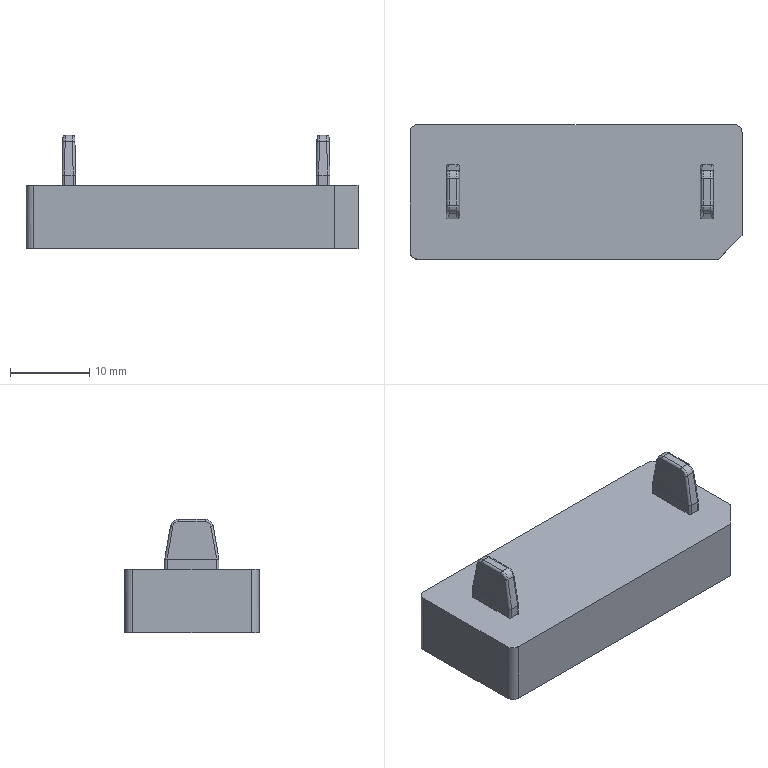NC program | PowerMill | posted by the shop | part box 42 x 17 x 14.346 mm
Lines 1 to 1529 of 50900:
%
G40 G49 G17 G80
( TOOL ID   D10C_1_1 )
( TOOL DIA. 10. TIP RAD 0 LENGTH 69.8 )
( Z = -.204 )
T1 M6
T3
G91 G28 Z0
G0 G90 G54
M08
S8000 M3
G0 X0 Y0 M8
G43 Z10.2 H1
X28.65 Y11.15
Z1.198
G1 Z-.002 F6000
X23.65 F10000
X-23.65
Y5.575
X23.65
Y0
X-23.65
Y-5.575
X23.65
Y-11.15
X-23.65
X-28.65
Z-.204
X-23.65
X23.65
Y-5.575
X-23.65
Y0
X23.65
Y5.575
X-23.65
Y11.15
X23.65
X28.65
G0 Z10.2
X.5 Y0
Z9.796
X-29.349 Y-4.749
Z.562
G1 Z-.638 F6000
X-28.822 F10000
G3 X-24.074 Y-.001 I0 J4.747
G1 Y10.15
G2 X-23.074 Y11.15 I1. J0
G1 X24.074
G2 X25.074 Y10.15 I0 J-1.
G1 Y-.001
X22.484 Y0
Y-2.32
X22.396 Y-3.094
X22.199 Y-3.867
X21.769 Y-4.832
X21.395 Y-5.414
X20.996 Y-5.89
X20.691 Y-6.187
X20.222 Y-6.578
X19.621 Y-6.961
X19.449 Y-7.051
X18.676 Y-7.361
X17.902 Y-7.548
X17.129 Y-7.619
X15.582 Y-7.593
X14.808 Y-7.454
X14.035 Y-7.199
X13.539 Y-6.961
X13.262 Y-6.798
X12.488 Y-6.204
X11.765 Y-5.414
X11.292 Y-4.641
X10.961 Y-3.867
X10.763 Y-3.094
X10.676 Y-2.32
Y-.093
X4.957 Y-.038
X4.925 Y-3.441
G2 X2.91 Y-5.422 I-2. J.019
G1 X-2.008 Y-5.386
G2 X-3.993 Y-3.373 I.014 J2.
G1 X-3.949 Y3.423
G2 X-1.938 Y5.409 I2. J-.013
G1 X3. Y5.383
G2 X4.989 Y3.364 I-.011 J-2.
G1 X4.957 Y-.038
X10.676 Y-.093
X10.675 Y2.32
X10.758 Y3.094
X10.941 Y3.849
X11.272 Y4.641
X11.715 Y5.385
X12.427 Y6.187
X13.262 Y6.838
X14.035 Y7.238
X14.808 Y7.493
X15.582 Y7.632
X17.129 Y7.659
X17.902 Y7.588
X18.676 Y7.401
X19.449 Y7.091
X19.692 Y6.961
X20.222 Y6.617
X20.733 Y6.187
X20.996 Y5.93
X21.424 Y5.414
X21.769 Y4.87
X21.888 Y4.641
X22.212 Y3.867
X22.402 Y3.094
X22.485 Y2.32
X22.484 Y0
X25.074 Y-.001
Y-10.15
G2 X24.074 Y-11.15 I-1. J0
G1 X-23.074
G2 X-24.074 Y-10.15 I0 J1.
G1 Y-.001
X-21.485 Y0
X-21.486 Y2.32
X-21.403 Y3.094
X-21.212 Y3.867
X-20.887 Y4.641
X-20.769 Y4.87
X-20.424 Y5.414
X-19.996 Y5.93
X-19.733 Y6.187
X-19.222 Y6.617
X-18.692 Y6.961
X-18.449 Y7.091
X-17.676 Y7.401
X-16.902 Y7.588
X-16.129 Y7.659
X-14.582 Y7.632
X-13.808 Y7.493
X-13.035 Y7.238
X-12.262 Y6.838
X-11.488 Y6.244
X-10.736 Y5.414
X-10.272 Y4.641
X-9.947 Y3.867
X-9.758 Y3.094
X-9.675 Y2.32
X-9.677 Y-2.32
X-9.763 Y-3.094
X-9.941 Y-3.809
X-10.292 Y-4.641
X-10.715 Y-5.346
X-11.469 Y-6.187
X-12.262 Y-6.798
X-12.538 Y-6.961
X-13.035 Y-7.198
X-13.808 Y-7.454
X-14.582 Y-7.593
X-16.129 Y-7.619
X-16.902 Y-7.548
X-17.676 Y-7.361
X-18.449 Y-7.051
X-19.222 Y-6.578
X-19.69 Y-6.187
X-19.996 Y-5.89
X-20.395 Y-5.414
X-20.769 Y-4.832
X-21.199 Y-3.867
X-21.397 Y-3.094
X-21.484 Y-2.32
X-21.485 Y0
X-24.074 Y-.001
G0 Z3.228
G1 X-29.349 Y-4.749
G0 Z.178
G1 Z-1.022 F6000
X-28.822 F10000
G3 X-24.074 Y-.001 I0 J4.747
G1 Y10.15
G2 X-23.074 Y11.15 I1. J0
G1 X24.074
G2 X25.074 Y10.15 I0 J-1.
G1 Y0
X22.5
Y-2.32
X22.445 Y-3.094
X22.283 Y-3.867
X21.995 Y-4.641
X21.769 Y-5.069
X21.553 Y-5.414
X20.996 Y-6.113
X20.222 Y-6.779
X19.954 Y-6.961
X19.449 Y-7.248
X18.676 Y-7.556
X17.924 Y-7.734
X17.129 Y-7.808
X15.582 Y-7.782
X14.808 Y-7.645
X14.035 Y-7.395
X13.262 Y-6.997
X12.488 Y-6.425
X12.237 Y-6.187
X11.715 Y-5.57
X11.165 Y-4.641
X10.877 Y-3.867
X10.715 Y-3.094
X10.66 Y-2.32
Y-.048
X4.896 Y-.019
X4.879 Y-3.412
G2 X2.879 Y-5.401 I-2. J.01
G1 X-1.878 Y-5.402
G2 X-3.878 Y-3.412 I0 J2.
G1 X-3.913 Y3.373
G2 X-1.913 Y5.383 I2. J.01
G1 X2.913
G2 X4.913 Y3.373 I0 J-2.
G1 X4.896 Y-.019
X10.66 Y-.048
X10.659 Y2.32
X10.709 Y3.094
X10.868 Y3.867
X10.941 Y4.117
X11.147 Y4.641
X11.581 Y5.414
X11.715 Y5.609
X12.199 Y6.187
X12.488 Y6.464
X13.142 Y6.961
X14.035 Y7.434
X14.808 Y7.684
X15.582 Y7.821
X17.129 Y7.847
X17.902 Y7.777
X18.676 Y7.596
X19.449 Y7.287
X20.222 Y6.821
X20.961 Y6.187
X21.579 Y5.414
X21.769 Y5.113
X22.013 Y4.641
X22.292 Y3.867
X22.452 Y3.094
X22.5 Y2.32
Y0
X25.074
Y-10.15
G2 X24.074 Y-11.15 I-1. J0
G1 X-23.074
G2 X-24.074 Y-10.15 I0 J1.
G1 Y-2.32
X-21.501
Y2.32
X-21.451 Y3.094
X-21.294 Y3.867
X-21.013 Y4.641
X-20.769 Y5.113
X-20.579 Y5.414
X-19.996 Y6.152
X-19.222 Y6.821
X-18.449 Y7.287
X-17.676 Y7.596
X-16.902 Y7.777
X-16.129 Y7.847
X-14.582 Y7.821
X-13.808 Y7.684
X-13.035 Y7.434
X-12.262 Y7.036
X-11.488 Y6.464
X-11.199 Y6.187
X-10.715 Y5.609
X-10.581 Y5.414
X-10.147 Y4.641
X-9.941 Y4.117
X-9.868 Y3.867
X-9.708 Y3.094
X-9.66 Y2.32
Y-2.32
X-9.715 Y-3.094
X-9.877 Y-3.867
X-10.165 Y-4.641
X-10.715 Y-5.57
X-11.237 Y-6.187
X-11.488 Y-6.425
X-12.206 Y-6.961
X-13.035 Y-7.395
X-13.808 Y-7.645
X-14.237 Y-7.734
X-14.582 Y-7.782
X-16.129 Y-7.808
X-16.902 Y-7.737
X-17.676 Y-7.556
X-18.449 Y-7.248
X-18.954 Y-6.961
X-19.222 Y-6.779
X-19.923 Y-6.187
X-20.553 Y-5.414
X-20.769 Y-5.069
X-20.995 Y-4.641
X-21.283 Y-3.867
X-21.446 Y-3.094
X-21.501 Y-2.32
X-24.074
Y-.001
G0 Z2.844
G1 X-29.349 Y-4.749
G0 Z-.206
G1 Z-1.406 F6000
X-28.822 F10000
G3 X-24.074 Y-.001 I0 J4.747
G1 Y10.15
G2 X-23.074 Y11.15 I1. J0
G1 X24.074
G2 X25.074 Y10.15 I0 J-1.
G1 Y0
X22.507
Y-2.32
X22.463 Y-3.094
X22.303 Y-3.867
X22.036 Y-4.641
X21.769 Y-5.167
X21.616 Y-5.414
X20.991 Y-6.187
X20.222 Y-6.866
X19.449 Y-7.327
X18.676 Y-7.627
X18.278 Y-7.734
X17.902 Y-7.812
X17.129 Y-7.881
X15.582 Y-7.855
X14.881 Y-7.734
X14.035 Y-7.47
X13.262 Y-7.081
X13.074 Y-6.961
X12.488 Y-6.501
X12.169 Y-6.187
X11.715 Y-5.657
X11.544 Y-5.414
X11.124 Y-4.641
X10.856 Y-3.867
X10.697 Y-3.094
X10.653 Y-2.32
Y2.32
X10.692 Y3.094
X10.846 Y3.867
X10.941 Y4.198
X11.108 Y4.641
X11.518 Y5.414
X11.715 Y5.697
X12.13 Y6.187
X12.488 Y6.54
X13.018 Y6.961
X13.262 Y7.121
X14.035 Y7.509
X14.731 Y7.734
X15.582 Y7.894
X17.129 Y7.92
X17.902 Y7.851
X18.676 Y7.666
X19.449 Y7.366
X20.142 Y6.961
X20.996 Y6.222
X21.641 Y5.414
X21.769 Y5.207
X22.053 Y4.641
X22.314 Y3.867
X22.467 Y3.094
X22.507 Y2.32
Y0
X25.074
Y-10.15
G2 X24.074 Y-11.15 I-1. J0
G1 X-23.074
G2 X-24.074 Y-10.15 I0 J1.
G1 Y-2.757
X-21.491 Y-2.61
X-21.507 Y-2.32
Y2.32
X-21.468 Y3.094
X-21.314 Y3.867
X-21.053 Y4.641
X-20.769 Y5.207
X-20.642 Y5.414
X-20.03 Y6.187
X-19.222 Y6.905
X-18.449 Y7.366
X-17.676 Y7.666
X-16.902 Y7.851
X-16.129 Y7.92
X-14.582 Y7.894
X-13.808 Y7.755
X-13.035 Y7.509
X-12.262 Y7.121
X-12.018 Y6.961
X-11.488 Y6.54
X-11.131 Y6.187
X-10.715 Y5.697
X-10.519 Y5.414
X-10.107 Y4.641
X-9.941 Y4.198
X-9.846 Y3.867
X-9.692 Y3.094
X-9.653 Y2.32
Y.002
X-3.902 Y-.001
X-3.901 Y3.379
G2 X-1.901 Y5.378 I2. J-.001
G1 X2.901 Y5.377
G2 X4.901 Y3.379 I0 J-2.
G1 X4.904 Y-3.38
G2 X2.904 Y-5.381 I-2. J-.001
G1 X-1.904
G2 X-3.904 Y-3.38 I0 J2.
G1 X-3.902 Y-.001
X-9.653 Y.002
Y-2.32
X-9.697 Y-3.094
X-9.856 Y-3.867
X-9.941 Y-4.159
X-10.124 Y-4.641
X-10.544 Y-5.414
X-10.715 Y-5.657
X-11.169 Y-6.187
X-11.488 Y-6.501
X-12.075 Y-6.961
X-12.262 Y-7.081
X-13.035 Y-7.47
X-13.882 Y-7.734
X-14.582 Y-7.855
X-16.129 Y-7.881
X-16.902 Y-7.812
X-17.676 Y-7.627
X-18.449 Y-7.327
X-19.222 Y-6.866
X-19.992 Y-6.187
X-20.617 Y-5.414
X-20.769 Y-5.167
X-21.036 Y-4.641
X-21.303 Y-3.867
X-21.463 Y-3.094
X-21.491 Y-2.61
X-24.074 Y-2.757
Y-.001
G0 Z2.459
G1 X-29.349 Y-4.749
G0 Z-.591
G1 Z-1.791 F6000
X-28.822 F10000
G3 X-24.074 Y-.001 I0 J4.747
G1 Y0
X-21.514
Y2.32
X-21.482 Y3.094
X-21.337 Y3.867
X-21.088 Y4.641
X-20.769 Y5.286
X-20.099 Y6.187
X-19.245 Y6.961
X-18.449 Y7.437
X-17.68 Y7.734
X-16.902 Y7.92
X-16.129 Y7.988
X-14.582 Y7.963
X-13.808 Y7.825
X-13.035 Y7.58
X-12.262 Y7.192
X-11.916 Y6.961
X-11.488 Y6.614
X-11.06 Y6.187
X-10.715 Y5.774
X-10.469 Y5.414
X-10.072 Y4.641
X-9.941 Y4.286
X-9.822 Y3.867
X-9.677 Y3.094
X-9.646 Y2.32
Y-.027
X-3.879 Y-.013
X-3.887 Y3.366
G2 X-1.892 Y5.371 I2. J.005
G1 X2.862 Y5.383
G2 X4.867 Y3.39 I.005 J-2.
G1 X4.891 Y-3.368
G2 X2.897 Y-5.375 I-2. J-.007
G1 X-1.865 Y-5.388
G2 X-3.871 Y-3.392 I-.005 J2.
G1 X-3.879 Y-.013
X-9.646 Y-.027
Y-2.32
X-9.682 Y-3.094
X-9.832 Y-3.867
X-9.941 Y-4.246
X-10.088 Y-4.641
X-10.494 Y-5.414
X-10.715 Y-5.734
X-11.098 Y-6.187
X-11.488 Y-6.575
X-11.97 Y-6.961
X-12.262 Y-7.153
X-13.035 Y-7.541
X-13.618 Y-7.734
X-14.582 Y-7.923
X-16.129 Y-7.949
X-16.902 Y-7.88
X-17.541 Y-7.734
X-18.449 Y-7.398
X-19.189 Y-6.961
X-19.996 Y-6.258
X-20.666 Y-5.414
X-21.072 Y-4.641
X-21.327 Y-3.867
X-21.478 Y-3.094
X-21.514 Y-2.32
Y0
X-24.074
Y10.15
G2 X-23.074 Y11.15 I1. J0
G1 X24.074
G2 X25.074 Y10.15 I0 J-1.
G1 Y2.522
X22.51 Y2.417
X22.514 Y2.32
Y-2.32
X22.478 Y-3.094
X22.328 Y-3.867
X22.071 Y-4.641
X21.666 Y-5.414
X21.063 Y-6.187
X20.222 Y-6.938
X19.449 Y-7.398
X18.541 Y-7.734
X17.902 Y-7.88
X17.129 Y-7.949
X15.582 Y-7.923
X14.808 Y-7.785
X14.035 Y-7.541
X13.262 Y-7.153
X12.97 Y-6.961
X12.488 Y-6.575
X12.097 Y-6.187
X11.715 Y-5.734
X11.494 Y-5.414
X11.088 Y-4.641
X10.941 Y-4.246
X10.833 Y-3.867
X10.682 Y-3.094
X10.646 Y-2.32
Y2.32
X10.678 Y3.094
X10.822 Y3.867
X10.941 Y4.286
X11.073 Y4.641
X11.469 Y5.414
X11.715 Y5.774
X12.061 Y6.187
X12.488 Y6.614
X12.915 Y6.961
X13.262 Y7.192
X14.035 Y7.58
X14.808 Y7.825
X15.582 Y7.963
X17.129 Y7.988
X17.902 Y7.92
X18.676 Y7.736
X19.449 Y7.437
X20.222 Y6.977
X20.996 Y6.297
X21.691 Y5.414
X22.088 Y4.641
X22.338 Y3.867
X22.482 Y3.094
X22.51 Y2.417
X25.074 Y2.522
Y-10.15
G2 X24.074 Y-11.15 I-1. J0
G1 X-23.074
G2 X-24.074 Y-10.15 I0 J1.
G1 Y-.001
G0 Z2.075
G1 X-29.349 Y-4.749
G0 Z-.975
G1 Z-2.175 F6000
X-28.822 F10000
G3 X-24.074 Y-.001 I0 J4.747
G1 Y0
X-21.521
Y2.32
X-21.497 Y3.094
X-21.361 Y3.867
X-21.122 Y4.641
X-20.769 Y5.365
X-20.169 Y6.187
X-19.996 Y6.371
X-19.342 Y6.961
X-18.449 Y7.508
X-17.898 Y7.734
X-16.902 Y7.988
X-16.129 Y8.056
X-14.582 Y8.031
X-13.808 Y7.894
X-13.035 Y7.65
X-12.262 Y7.264
X-11.817 Y6.961
X-11.488 Y6.687
X-10.992 Y6.187
X-10.715 Y5.85
X-10.42 Y5.414
X-10.038 Y4.641
X-9.798 Y3.867
X-9.664 Y3.094
X-9.639 Y2.32
Y-.027
X-3.866 Y-.013
X-3.874 Y3.359
G2 X-1.879 Y5.364 I2. J.005
G1 X2.85 Y5.376
G2 X4.854 Y3.383 I.005 J-2.
G1 X4.878 Y-3.361
G2 X2.883 Y-5.368 I-2. J-.007
G1 X-1.853 Y-5.38
G2 X-3.858 Y-3.385 I-.005 J2.
G1 X-3.866 Y-.013
X-9.639 Y-.027
Y-2.32
X-9.667 Y-3.094
X-9.808 Y-3.867
X-10.054 Y-4.641
X-10.444 Y-5.414
X-10.715 Y-5.81
X-11.027 Y-6.187
X-11.488 Y-6.648
X-11.869 Y-6.961
X-12.262 Y-7.225
X-13.035 Y-7.611
X-13.381 Y-7.734
X-13.808 Y-7.855
X-14.582 Y-7.992
X-16.129 Y-8.017
X-16.902 Y-7.949
X-17.676 Y-7.766
X-18.449 Y-7.469
X-19.29 Y-6.961
X-20.133 Y-6.187
X-20.716 Y-5.414
X-21.106 Y-4.641
X-21.351 Y-3.867
X-21.493 Y-3.094
X-21.521 Y-2.32
Y0
X-24.074
Y10.15
G2 X-23.074 Y11.15 I1. J0
G1 X24.074
G2 X25.074 Y10.15 I0 J-1.
G1 Y3.173
X22.497 Y3.094
X22.521 Y2.32
Y-2.32
X22.493 Y-3.094
X22.352 Y-3.867
X22.106 Y-4.641
X21.769 Y-5.325
X21.132 Y-6.187
X20.291 Y-6.961
X19.449 Y-7.469
X18.779 Y-7.734
X17.902 Y-7.949
X17.129 Y-8.017
X15.582 Y-7.992
X14.808 Y-7.855
X14.035 Y-7.611
X13.262 Y-7.225
X12.87 Y-6.961
X12.488 Y-6.648
X12.027 Y-6.187
X11.715 Y-5.81
X11.444 Y-5.414
X11.054 Y-4.641
X10.809 Y-3.867
X10.667 Y-3.094
X10.639 Y-2.32
Y2.32
X10.663 Y3.094
X10.797 Y3.867
X11.038 Y4.641
X11.421 Y5.414
X11.715 Y5.85
X11.991 Y6.187
X12.488 Y6.687
X12.818 Y6.961
X13.262 Y7.264
X14.035 Y7.65
X14.808 Y7.894
X15.582 Y8.031
X17.129 Y8.056
X17.902 Y7.988
X18.676 Y7.805
X19.449 Y7.508
X20.222 Y7.05
X20.996 Y6.371
X21.168 Y6.187
X21.74 Y5.414
X22.122 Y4.641
X22.362 Y3.867
X22.497 Y3.094
X25.074 Y3.173
Y-10.15
G2 X24.074 Y-11.15 I-1. J0
G1 X-23.074
G2 X-24.074 Y-10.15 I0 J1.
G1 Y-.001
G0 Z1.691
G1 X-29.349 Y-4.749
G0 Z-1.359
G1 Z-2.559 F6000
X-28.822 F10000
G3 X-24.074 Y-.001 I0 J4.747
G1 Y0
X-21.527
Y2.32
X-21.509 Y3.094
X-21.385 Y3.867
X-21.154 Y4.641
X-20.787 Y5.414
X-20.234 Y6.187
X-19.996 Y6.446
X-19.436 Y6.961
X-19.222 Y7.122
X-18.449 Y7.579
X-18.089 Y7.734
X-17.676 Y7.875
X-16.902 Y8.057
X-16.129 Y8.124
X-14.582 Y8.099
X-13.808 Y7.964
X-13.07 Y7.734
X-12.262 Y7.336
X-11.725 Y6.961
X-11.488 Y6.761
X-10.926 Y6.187
X-10.715 Y5.927
X-10.374 Y5.414
X-10.006 Y4.641
X-9.774 Y3.867
X-9.651 Y3.094
X-9.633 Y2.32
Y.026
X-3.821 Y.007
X-3.809 Y3.388
G2 X-1.807 Y5.382 I2. J-.007
G1 X2.831 Y5.377
G2 X4.829 Y3.388 I-.002 J-2.
G1 X4.865 Y-3.351
G2 X2.873 Y-5.362 I-2. J-.01
G1 X-1.823 Y-5.382
G2 X-3.832 Y-3.375 I-.008 J2.
G1 X-3.821 Y.007
X-9.633 Y.026
Y-2.32
X-9.655 Y-3.094
X-9.784 Y-3.867
X-10.021 Y-4.641
X-10.397 Y-5.414
X-10.715 Y-5.887
X-10.96 Y-6.187
X-11.488 Y-6.722
X-11.774 Y-6.961
X-12.262 Y-7.297
X-13.175 Y-7.734
X-13.808 Y-7.924
X-14.582 Y-8.06
X-16.129 Y-8.084
X-16.902 Y-8.018
X-17.676 Y-7.836
X-17.986 Y-7.734
X-18.449 Y-7.54
X-19.222 Y-7.083
X-19.386 Y-6.961
X-19.996 Y-6.407
X-20.199 Y-6.187
X-20.763 Y-5.414
X-21.139 Y-4.641
X-21.375 Y-3.867
X-21.506 Y-3.094
X-21.527 Y-2.32
Y0
X-24.074
Y10.15
G2 X-23.074 Y11.15 I1. J0
G1 X24.074
G2 X25.074 Y10.15 I0 J-1.
G1 Y3.155
X22.509 Y3.094
X22.527 Y2.32
Y-2.32
X22.506 Y-3.094
X22.376 Y-3.867
X22.139 Y-4.641
X21.769 Y-5.404
X21.2 Y-6.187
X20.996 Y-6.407
X20.386 Y-6.961
X20.222 Y-7.083
X19.449 Y-7.54
X18.985 Y-7.734
X18.676 Y-7.836
X17.902 Y-8.018
X17.129 Y-8.084
X15.582 Y-8.06
X14.808 Y-7.924
X14.174 Y-7.734
X13.262 Y-7.297
X12.774 Y-6.961
X12.488 Y-6.722
X11.96 Y-6.187
X11.715 Y-5.887
X11.397 Y-5.414
X11.02 Y-4.641
X10.785 Y-3.867
X10.654 Y-3.094
X10.633 Y-2.32
Y2.32
X10.651 Y3.094
X10.775 Y3.867
X11.005 Y4.641
X11.373 Y5.414
X11.715 Y5.927
X11.926 Y6.187
X12.488 Y6.761
X12.724 Y6.961
X13.262 Y7.336
X14.035 Y7.721
X14.808 Y7.964
X15.582 Y8.099
X17.129 Y8.124
X17.902 Y8.057
X18.676 Y7.875
X19.089 Y7.734
X19.449 Y7.579
X20.222 Y7.122
X20.435 Y6.961
X20.996 Y6.446
X21.234 Y6.187
X21.769 Y5.444
X22.154 Y4.641
X22.386 Y3.867
X22.509 Y3.094
X25.074 Y3.155
Y-10.15
G2 X24.074 Y-11.15 I-1. J0
G1 X-23.074
G2 X-24.074 Y-10.15 I0 J1.
G1 Y-.001
G0 Z1.307
G1 X-29.349 Y-4.749
G0 Z-1.743
G1 Z-2.943 F6000
X-28.822 F10000
G3 X-24.074 Y-.001 I0 J4.747
G1 Y10.15
G2 X-23.074 Y11.15 I1. J0
G1 X24.074
G2 X25.074 Y10.15 I0 J-1.
G1 Y3.138
X22.521 Y3.094
X22.534 Y2.32
X22.527 Y.081
Y-2.32
X22.519 Y-2.608
X22.518 Y-3.094
X22.399 Y-3.867
X22.172 Y-4.641
X21.81 Y-5.414
X21.266 Y-6.187
X20.996 Y-6.481
X20.478 Y-6.961
X20.222 Y-7.156
X19.449 Y-7.611
X19.168 Y-7.734
X18.676 Y-7.906
X17.902 Y-8.087
X17.129 Y-8.152
X15.582 Y-8.128
X14.808 Y-7.994
X14.035 Y-7.752
X13.262 Y-7.368
X12.682 Y-6.961
X12.488 Y-6.796
X11.894 Y-6.187
X11.715 Y-5.964
X11.351 Y-5.414
X10.988 Y-4.641
X10.761 Y-3.867
X10.643 Y-3.094
X10.626 Y-2.32
X10.633 Y.302
Y2.32
X10.638 Y2.56
X10.64 Y3.094
X10.752 Y3.867
X10.941 Y4.549
X11.328 Y5.414
X11.715 Y6.003
X11.861 Y6.187
X12.488 Y6.835
X13.262 Y7.408
X13.898 Y7.734
X14.808 Y8.033
X15.582 Y8.168
X17.129 Y8.191
X17.902 Y8.126
X18.676 Y7.945
X19.449 Y7.65
X20.222 Y7.195
X20.526 Y6.961
X20.996 Y6.52
X21.298 Y6.187
X21.769 Y5.522
X22.186 Y4.641
X22.408 Y3.867
X22.521 Y3.094
X25.074 Y3.138
Y-10.15
G2 X24.074 Y-11.15 I-1. J0
G1 X-23.074
G2 X-24.074 Y-10.15 I0 J1.
G1 Y-1.008
X-21.531 Y-1.014
X-21.527 Y.292
Y2.32
X-21.522 Y2.564
X-21.52 Y3.094
X-21.408 Y3.867
X-21.187 Y4.641
X-20.832 Y5.414
X-20.299 Y6.187
X-19.996 Y6.52
X-19.526 Y6.961
X-19.222 Y7.195
X-18.449 Y7.65
X-17.676 Y7.945
X-16.902 Y8.126
X-16.129 Y8.191
X-14.582 Y8.168
X-13.808 Y8.033
X-13.035 Y7.791
X-12.262 Y7.408
X-11.634 Y6.961
X-10.861 Y6.187
X-10.715 Y6.003
X-10.327 Y5.414
X-9.974 Y4.641
X-9.752 Y3.867
X-9.638 Y3.094
X-9.626 Y2.32
X-9.633 Y.13
Y-.051
X-3.831 Y-.023
X-3.847 Y3.342
G2 X-1.857 Y5.352 I2. J.01
G1 X2.803 Y5.374
G2 X4.812 Y3.386 I.009 J-2.
G1 X4.851 Y-3.344
G2 X2.861 Y-5.355 I-2. J-.012
G1 X-1.804 Y-5.378
G2 X-3.814 Y-3.388 I-.01 J2.
G1 X-3.831 Y-.023
X-9.633 Y-.051
Y-2.32
X-9.641 Y-2.618
X-9.643 Y-3.094
X-9.761 Y-3.867
X-9.941 Y-4.51
X-10.35 Y-5.414
X-10.715 Y-5.964
X-10.894 Y-6.187
X-11.488 Y-6.796
X-11.682 Y-6.961
X-12.262 Y-7.368
X-12.992 Y-7.734
X-13.808 Y-7.994
X-14.582 Y-8.128
X-16.129 Y-8.152
X-16.902 Y-8.087
X-17.676 Y-7.906
X-18.168 Y-7.734
X-18.449 Y-7.611
X-19.222 Y-7.156
X-19.478 Y-6.961
X-19.996 Y-6.481
X-20.266 Y-6.187
X-20.769 Y-5.483
X-21.173 Y-4.641
X-21.399 Y-3.867
X-21.517 Y-3.094
X-21.534 Y-2.32
X-21.531 Y-1.014
X-24.074 Y-1.008
Y-.001
G0 Z.923
G1 X-29.349 Y-4.749
G0 Z-2.127
G1 Z-3.327 F6000
X-28.822 F10000
G3 X-24.074 Y-.001 I0 J4.747
G1 Y10.15
G2 X-23.074 Y11.15 I1. J0
G1 X24.074
G2 X25.074 Y10.15 I0 J-1.
G1 Y-.742
X22.531 Y-.741
X22.53 Y-3.094
X22.421 Y-3.867
X22.203 Y-4.641
X21.854 Y-5.414
X21.329 Y-6.187
X20.996 Y-6.556
X20.567 Y-6.961
X20.222 Y-7.228
X19.335 Y-7.734
X18.676 Y-7.975
X17.902 Y-8.156
X17.129 Y-8.22
X15.582 Y-8.197
X14.808 Y-8.063
X14.035 Y-7.822
X13.262 Y-7.44
X12.594 Y-6.961
X11.831 Y-6.187
X11.305 Y-5.414
X10.957 Y-4.641
X10.739 Y-3.867
X10.631 Y-3.094
X10.63 Y-2.534
X10.626 Y-2.32
X10.63 Y-.793
X10.628 Y3.094
X10.73 Y3.867
X10.941 Y4.637
X11.283 Y5.414
X11.715 Y6.08
X12.488 Y6.909
X13.262 Y7.48
X13.74 Y7.734
X14.035 Y7.861
X14.808 Y8.102
X15.582 Y8.236
X17.129 Y8.259
X17.902 Y8.195
X18.676 Y8.014
X19.42 Y7.734
X20.222 Y7.267
X20.612 Y6.961
X20.996 Y6.595
X21.36 Y6.187
X21.769 Y5.601
X21.876 Y5.414
X22.217 Y4.641
X22.429 Y3.867
X22.533 Y3.094
X22.532 Y2.424
X22.534 Y2.32
X22.532 Y1.612
X22.531 Y-.741
X25.074 Y-.742
Y-10.15
G2 X24.074 Y-11.15 I-1. J0
G1 X-23.074
G2 X-24.074 Y-10.15 I0 J1.
G1 Y-3.095
X-21.529 Y-3.094
Y-2.544
X-21.534 Y-2.32
X-21.53 Y-.724
X-21.532 Y3.094
X-21.429 Y3.867
X-21.217 Y4.641
X-20.876 Y5.414
X-20.361 Y6.187
X-19.996 Y6.595
X-19.612 Y6.961
X-19.222 Y7.267
X-18.449 Y7.721
X-17.676 Y8.014
X-16.902 Y8.195
X-16.129 Y8.259
X-14.582 Y8.236
X-13.808 Y8.102
X-13.035 Y7.861
X-12.74 Y7.734
X-12.262 Y7.48
X-11.548 Y6.961
X-10.799 Y6.187
X-10.284 Y5.414
X-9.942 Y4.641
X-9.731 Y3.867
X-9.628 Y3.094
X-9.629 Y2.483
X-9.626 Y2.32
X-9.629 Y1.327
Y-.057
X-3.821 Y-.025
X-3.84 Y3.333
G2 X-1.85 Y5.344 I2. J.011
G1 X2.791 Y5.367
G2 X4.801 Y3.38 I.01 J-2.
G1 X4.844 Y-3.333
G2 X2.855 Y-5.346 I-2. J-.013
G1 X-1.792 Y-5.372
G2 X-3.803 Y-3.383 I-.011 J2.
G1 X-3.821 Y-.025
X-9.629 Y-.057
X-9.63 Y-3.094
X-9.74 Y-3.867
X-9.941 Y-4.598
X-10.306 Y-5.414
X-10.831 Y-6.187
X-11.488 Y-6.869
X-12.262 Y-7.44
X-12.825 Y-7.734
X-13.035 Y-7.822
X-13.808 Y-8.063
X-14.582 Y-8.197
X-16.129 Y-8.22
X-16.902 Y-8.156
X-17.676 Y-7.975
X-18.334 Y-7.734
X-19.222 Y-7.228
X-19.567 Y-6.961
X-19.996 Y-6.556
X-20.329 Y-6.187
X-20.769 Y-5.562
X-21.203 Y-4.641
X-21.421 Y-3.867
X-21.529 Y-3.094
X-24.074 Y-3.095
Y-.001
G0 Z.539
G1 X-29.349 Y-4.749
G0 Z-2.511
G1 Z-3.711 F6000
X-28.822 F10000
G3 X-24.074 Y-.001 I0 J4.747
G1 X-21.542 Y0
X-21.543 Y3.094
X-21.45 Y3.867
X-21.246 Y4.641
X-20.919 Y5.414
X-20.769 Y5.68
X-20.422 Y6.187
X-19.996 Y6.67
X-19.696 Y6.961
X-19.222 Y7.34
X-18.566 Y7.734
X-17.676 Y8.084
X-16.902 Y8.264
X-16.129 Y8.327
X-14.582 Y8.304
X-13.808 Y8.172
X-13.035 Y7.932
X-12.593 Y7.734
X-12.262 Y7.551
X-11.488 Y6.982
X-10.739 Y6.187
X-10.241 Y5.414
X-9.941 Y4.724
X-9.711 Y3.867
X-9.619 Y3.094
Y-.051
X-3.809 Y-.022
X-3.825 Y3.33
G2 X-1.834 Y5.34 I2. J.01
G1 X2.782 Y5.361
G2 X4.791 Y3.373 I.009 J-2.
G1 X4.828 Y-3.332
G2 X2.838 Y-5.343 I-2. J-.011
G1 X-1.783 Y-5.365
G2 X-3.793 Y-3.375 I-.01 J2.
G1 X-3.809 Y-.022
X-9.619 Y-.051
Y-3.094
X-9.719 Y-3.867
X-9.926 Y-4.641
X-10.262 Y-5.414
X-10.715 Y-6.117
X-11.488 Y-6.943
X-12.262 Y-7.512
X-12.673 Y-7.734
X-13.035 Y-7.892
X-13.808 Y-8.133
X-14.582 Y-8.265
X-16.129 Y-8.288
X-16.902 Y-8.224
X-17.676 Y-8.045
X-18.449 Y-7.753
X-19.222 Y-7.301
X-19.651 Y-6.961
X-19.996 Y-6.63
X-20.391 Y-6.187
X-20.769 Y-5.641
X-20.898 Y-5.414
X-21.233 Y-4.641
X-21.442 Y-3.867
X-21.541 Y-3.094
X-21.542 Y0
X-24.074 Y-.001
Y10.15
G2 X-23.074 Y11.15 I1. J0
G1 X24.074
G2 X25.074 Y10.15 I0 J-1.
G1 Y.001
X22.542 Y.002
X22.541 Y-3.094
X22.442 Y-3.867
X22.233 Y-4.641
X21.898 Y-5.414
X21.769 Y-5.641
X21.39 Y-6.187
X20.996 Y-6.63
X20.651 Y-6.961
X20.222 Y-7.301
X19.487 Y-7.734
X18.676 Y-8.045
X17.902 Y-8.224
X17.129 Y-8.288
X15.582 Y-8.265
X14.808 Y-8.133
X14.035 Y-7.892
X13.673 Y-7.734
X13.262 Y-7.512
X12.488 Y-6.943
X11.769 Y-6.187
X11.262 Y-5.414
X10.941 Y-4.685
X10.718 Y-3.867
X10.619 Y-3.094
X10.618 Y3.094
X10.71 Y3.867
X10.913 Y4.641
X11.241 Y5.414
X11.715 Y6.157
X12.464 Y6.961
X13.262 Y7.551
X13.593 Y7.734
X14.035 Y7.932
X14.808 Y8.172
X15.582 Y8.304
X17.129 Y8.327
X17.902 Y8.264
X18.676 Y8.084
X19.449 Y7.792
X20.222 Y7.34
X20.695 Y6.961
X20.996 Y6.67
X21.421 Y6.187
X21.769 Y5.68
X21.919 Y5.414
X22.246 Y4.641
X22.45 Y3.867
X22.543 Y3.097
X22.542 Y.002
X25.074 Y.001
Y-10.15
G2 X24.074 Y-11.15 I-1. J0
G1 X-23.074
G2 X-24.074 Y-10.15 I0 J1.
G1 Y-.001
G0 Z.155
G1 X-29.349 Y-4.749
G0 Z-2.895
G1 Z-4.095 F6000
X-28.822 F10000
G3 X-24.074 Y-.001 I0 J4.747
G1 Y10.15
G2 X-23.074 Y11.15 I1. J0
G1 X24.074
G2 X25.074 Y10.15 I0 J-1.
G1 Y.098
X22.546 Y.096
X22.55 Y-3.094
X22.462 Y-3.867
X22.263 Y-4.641
X21.941 Y-5.414
X21.769 Y-5.72
X21.45 Y-6.187
X20.996 Y-6.705
X20.734 Y-6.961
X20.222 Y-7.373
X19.629 Y-7.734
X19.449 Y-7.823
X18.676 Y-8.115
X17.902 Y-8.293
X17.129 Y-8.355
X15.582 Y-8.334
X14.808 Y-8.202
X14.035 Y-7.963
X13.531 Y-7.734
X13.262 Y-7.584
X12.488 Y-7.017
X11.715 Y-6.194
X11.22 Y-5.414
X10.941 Y-4.771
X10.697 Y-3.867
X10.61 Y-3.094
X10.609 Y3.094
X10.691 Y3.867
X10.884 Y4.641
X11.199 Y5.414
X11.681 Y6.187
X12.384 Y6.961
X13.262 Y7.623
X14.035 Y8.002
X14.808 Y8.241
X15.582 Y8.373
X17.129 Y8.395
X17.902 Y8.332
X18.676 Y8.154
X19.449 Y7.863
X19.703 Y7.734
X20.222 Y7.412
X20.776 Y6.961
X20.996 Y6.744
X21.479 Y6.187
X21.769 Y5.759
X21.961 Y5.414
X22.275 Y4.641
X22.469 Y3.867
X22.543 Y3.285
X22.546 Y.096
X25.074 Y.098
Y-10.15
G2 X24.074 Y-11.15 I-1. J0
G1 X-23.074
G2 X-24.074 Y-10.15 I0 J1.
G1 Y-.08
X-21.547 Y-.076
X-21.552 Y3.094
X-21.47 Y3.867
X-21.276 Y4.641
X-20.96 Y5.414
X-20.769 Y5.759
X-20.479 Y6.187
X-19.996 Y6.744
X-19.776 Y6.961
X-19.222 Y7.412
X-18.702 Y7.734
X-18.449 Y7.863
X-17.676 Y8.154
X-16.902 Y8.332
X-16.129 Y8.395
X-14.582 Y8.373
X-13.808 Y8.241
X-13.035 Y8.002
X-12.262 Y7.623
X-11.488 Y7.056
X-10.715 Y6.233
X-10.199 Y5.414
X-9.941 Y4.81
X-9.69 Y3.867
X-9.609 Y3.094
X-9.61 Y-.042
X-3.797 Y-.019
X-3.811 Y3.328
G2 X-1.819 Y5.336 I2. J.008
G1 X2.775 Y5.354
G2 X4.782 Y3.364 I.008 J-2.
G1 X4.815 Y-3.329
G2 X2.823 Y-5.339 I-2. J-.01
G1 X-1.776 Y-5.358
G2 X-3.784 Y-3.366 I-.008 J2.
G1 X-3.797 Y-.019
X-9.61 Y-.042
X-9.611 Y-3.094
X-9.698 Y-3.867
X-9.898 Y-4.641
X-10.219 Y-5.414
X-10.711 Y-6.187
X-11.426 Y-6.961
X-12.262 Y-7.584
X-12.531 Y-7.734
X-13.035 Y-7.963
X-13.808 Y-8.202
X-14.582 Y-8.334
X-16.129 Y-8.355
X-16.902 Y-8.293
X-17.676 Y-8.115
X-18.449 Y-7.823
X-19.222 Y-7.373
X-19.733 Y-6.961
X-19.996 Y-6.705
X-20.45 Y-6.187
X-20.769 Y-5.72
X-20.94 Y-5.414
X-21.263 Y-4.641
X-21.463 Y-3.867
X-21.543 Y-3.246
X-21.547 Y-.076
X-24.074 Y-.08
Y-.001
G0 Z-.229
G1 X-29.349 Y-4.749
G0 Z-3.279
G1 Z-4.479 F6000
X-28.822 F10000
G3 X-24.074 Y-.001 I0 J4.747
G1 Y10.15
G2 X-23.074 Y11.15 I1. J0
G1 X24.074
G2 X25.074 Y10.15 I0 J-1.
G1 Y0
X22.559
Y-3.094
X22.48 Y-3.867
X22.291 Y-4.641
X21.981 Y-5.414
X21.769 Y-5.799
X21.507 Y-6.187
X20.996 Y-6.779
X20.812 Y-6.961
X20.222 Y-7.446
X19.761 Y-7.734
X19.449 Y-7.894
X18.676 Y-8.184
X17.902 Y-8.362
X17.129 Y-8.423
X15.582 Y-8.402
X14.808 Y-8.271
X14.035 Y-8.033
X13.398 Y-7.734
X12.488 Y-7.091
X11.715 Y-6.27
X11.179 Y-5.414
X10.941 Y-4.858
X10.679 Y-3.867
X10.601 Y-3.094
X10.6 Y3.094
X10.672 Y3.867
X10.857 Y4.641
X10.941 Y4.897
X11.159 Y5.414
X11.623 Y6.187
X12.307 Y6.961
X12.488 Y7.13
X13.262 Y7.695
X14.035 Y8.072
X14.808 Y8.311
X15.582 Y8.441
X17.129 Y8.462
X17.902 Y8.401
X18.676 Y8.224
X19.449 Y7.934
X19.83 Y7.734
X20.222 Y7.485
X20.853 Y6.961
X21.537 Y6.187
X21.769 Y5.838
X22.001 Y5.414
X22.303 Y4.641
X22.488 Y3.867
X22.541 Y3.3
X22.543 Y3.285
Y3.279
X22.56 Y3.094
X22.559 Y0
X25.074
Y-10.15
G2 X24.074 Y-11.15 I-1. J0
G1 X-23.074
G2 X-24.074 Y-10.15 I0 J1.
G1 Y-3.094
X-21.559
X-21.56 Y3.094
X-21.543 Y3.441
X-21.488 Y3.867
X-21.303 Y4.641
X-21.001 Y5.414
X-20.769 Y5.838
X-20.537 Y6.187
X-19.996 Y6.819
X-19.222 Y7.485
X-18.83 Y7.734
X-18.449 Y7.934
X-17.676 Y8.224
X-16.902 Y8.401
X-16.129 Y8.462
X-14.582 Y8.441
X-13.808 Y8.311
X-13.035 Y8.072
X-12.329 Y7.734
X-11.488 Y7.13
X-11.307 Y6.961
X-10.715 Y6.31
X-10.159 Y5.414
X-9.857 Y4.641
X-9.672 Y3.867
X-9.6 Y3.094
X-9.601 Y-.036
X-3.787 Y-.016
X-3.798 Y3.326
G2 X-1.805 Y5.333 I2. J.007
G1 X2.767 Y5.348
G2 X4.774 Y3.356 I.006 J-2.
G1 X4.802 Y-3.327
G2 X2.809 Y-5.335 I-2. J-.008
G1 X-1.768 Y-5.351
G2 X-3.775 Y-3.358 I-.007 J2.
G1 X-3.787 Y-.016
X-9.601 Y-.036
X-9.602 Y-3.094
X-9.679 Y-3.867
X-9.869 Y-4.641
X-10.179 Y-5.414
X-10.715 Y-6.27
X-11.488 Y-7.091
X-12.262 Y-7.656
X-12.399 Y-7.734
X-13.035 Y-8.033
X-13.808 Y-8.271
X-14.582 Y-8.402
X-16.129 Y-8.423
X-16.902 Y-8.362
X-17.676 Y-8.184
X-18.449 Y-7.894
X-18.762 Y-7.734
X-19.222 Y-7.446
X-19.813 Y-6.961
X-20.508 Y-6.187
X-20.769 Y-5.799
X-20.981 Y-5.414